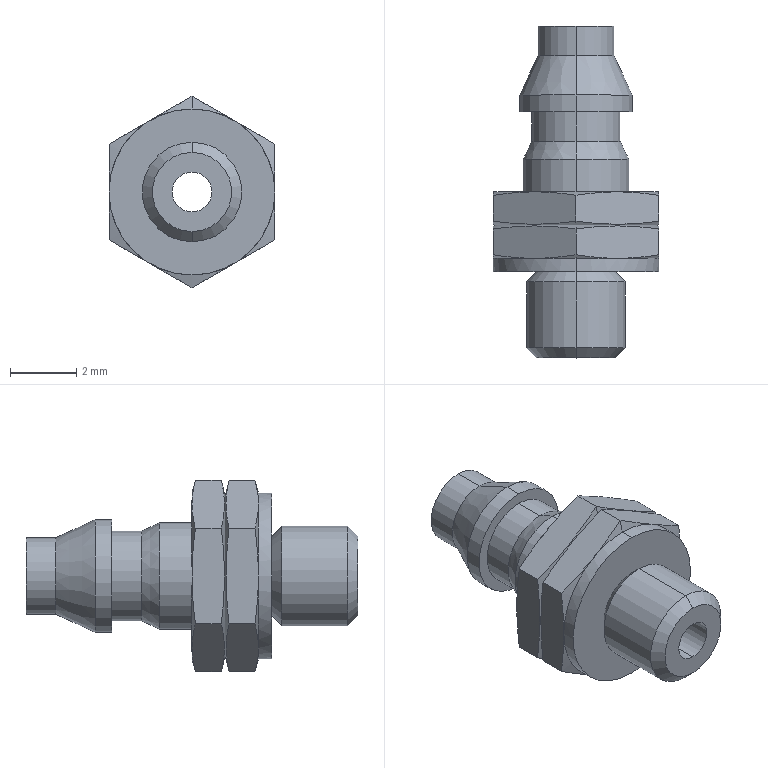Part | SolidWorks | features BaseBody 1 | 1 solid | 57 faces | box 5 x 10 x 5.774 mm | volume 89.646 mm3 | cone 26 | plane 17 | cylinder 14 | commonest cylinder face diameters 1.2 x2 2.3 x2 2.7 x2 3 x2 3.2 x2 3.4 x2